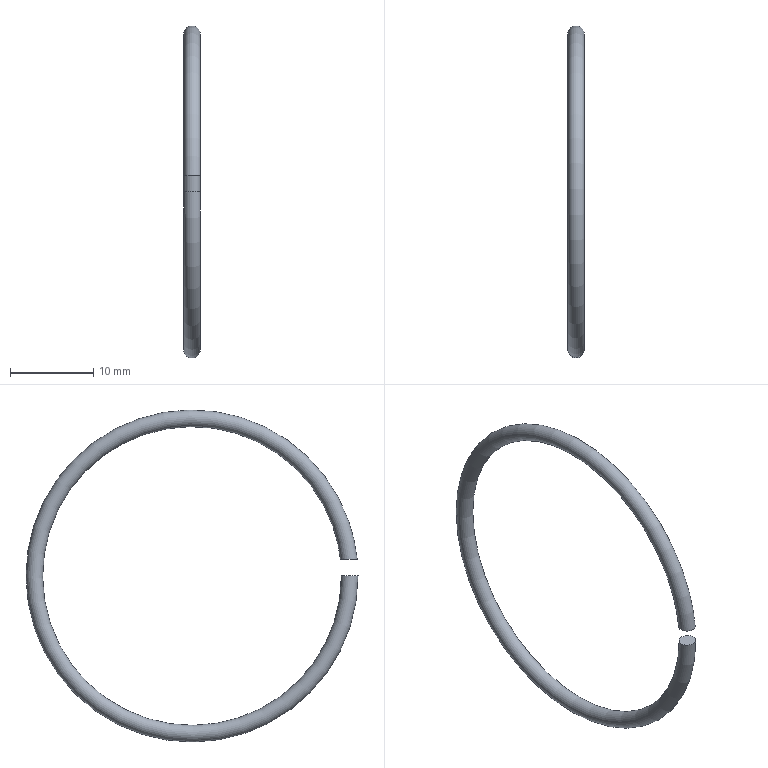Part | NX | features 1 2 | 1 solid | 3 faces | box 2 x 39.9 x 39.9 mm | volume 367.755 mm3 | plane 2 | torus 1
STEP:
#1=CARTESIAN_POINT('',(-1489.5,-459.849,-298.));
#2=VERTEX_POINT('',#1);
#3=CARTESIAN_POINT('',(-1488.714,-459.63,-298.));
#4=CARTESIAN_POINT('',(-1489.5,-459.959,-298.));
#5=CARTESIAN_POINT('',(-1490.285,-459.63,-298.));
#6=CARTESIAN_POINT('',(-1490.607,-458.845,-298.));
#7=CARTESIAN_POINT('',(-1490.286,-458.058,-298.));
#8=CARTESIAN_POINT('',(-1489.5,-457.728,-298.));
#9=CARTESIAN_POINT('',(-1488.715,-458.058,-298.));
#10=CARTESIAN_POINT('',(-1488.393,-458.843,-298.));
#11=CARTESIAN_POINT('',(-1488.714,-459.63,-298.));
#12=CARTESIAN_POINT('',(-1489.5,-459.959,-298.));
#13=CARTESIAN_POINT('',(-1490.285,-459.63,-298.));
#14=B_SPLINE_CURVE_WITH_KNOTS('',3,(#3,#4,#5,#6,#7,#8,#9,#10,#11,#12,#13),.UNSPECIFIED.,.T.,.F.,(1,1,1,1,1,1,1,1,1,1,1,1,1,1,1),(-0.002351,-0.001567,-0.0007837,0.,0.0007837,0.001567,0.002351,0.003135,0.003918,0.004702,0.005486,0.00627,0.007053,0.007837,0.008621),.UNSPECIFIED.);
#15=EDGE_CURVE('',#2,#2,#14,.T.);
#16=ORIENTED_EDGE('',*,*,#15,.F.);
#17=EDGE_LOOP('',(#16));
#18=FACE_BOUND('',#17,.T.);
#19=CARTESIAN_POINT('',(-1489.5,-459.95,-300.));
#20=VERTEX_POINT('',#19);
#21=CARTESIAN_POINT('',(-1489.5,-458.95,-300.));
#22=DIRECTION('',(0.,0.,1.));
#23=DIRECTION('',(0.,-1.,0.));
#24=AXIS2_PLACEMENT_3D('',#21,#22,#23);
#25=CIRCLE('',#24,1.);
#26=EDGE_CURVE('',#20,#20,#25,.T.);
#27=ORIENTED_EDGE('',*,*,#26,.F.);
#28=EDGE_LOOP('',(#27));
#29=FACE_BOUND('',#28,.T.);
#30=CARTESIAN_POINT('',(-1489.5,-440.,-300.));
#31=DIRECTION('',(1.,0.,0.));
#32=DIRECTION('',(0.,1.,0.));
#33=AXIS2_PLACEMENT_3D('',#30,#31,#32);
#34=TOROIDAL_SURFACE('',#33,18.95,1.);
#35=ADVANCED_FACE('',(#18,#29),#34,.T.);
#36=ORIENTED_EDGE('',*,*,#15,.T.);
#37=EDGE_LOOP('',(#36));
#38=FACE_BOUND('',#37,.T.);
#39=CARTESIAN_POINT('',(-1494.5,-456.95,-298.));
#40=DIRECTION('',(0.,0.,1.));
#41=DIRECTION('',(1.,0.,0.));
#42=AXIS2_PLACEMENT_3D('',#39,#40,#41);
#43=PLANE('',#42);
#44=ADVANCED_FACE('',(#38),#43,.F.);
#45=ORIENTED_EDGE('',*,*,#26,.T.);
#46=EDGE_LOOP('',(#45));
#47=FACE_BOUND('',#46,.T.);
#48=CARTESIAN_POINT('',(-1494.5,-461.95,-300.));
#49=DIRECTION('',(0.,0.,-1.));
#50=DIRECTION('',(-1.,0.,0.));
#51=AXIS2_PLACEMENT_3D('',#48,#49,#50);
#52=PLANE('',#51);
#53=ADVANCED_FACE('',(#47),#52,.F.);
#54=CLOSED_SHELL('',(#35,#44,#53));
#55=MANIFOLD_SOLID_BREP('',#54);
#56=(LENGTH_UNIT()NAMED_UNIT(*)SI_UNIT(.MILLI.,.METRE.));
#57=UNCERTAINTY_MEASURE_WITH_UNIT(LENGTH_MEASURE(0.0508),#56,'','');
#58=(NAMED_UNIT(*)PLANE_ANGLE_UNIT()SI_UNIT($,.RADIAN.));
#59=(NAMED_UNIT(*)SI_UNIT($,.STERADIAN.)SOLID_ANGLE_UNIT());
#60=(GEOMETRIC_REPRESENTATION_CONTEXT(3)GLOBAL_UNCERTAINTY_ASSIGNED_CONTEXT((#57))GLOBAL_UNIT_ASSIGNED_CONTEXT((#56,#58,#59))REPRESENTATION_CONTEXT('',''));
#61=ADVANCED_BREP_SHAPE_REPRESENTATION('',(#55),#60);